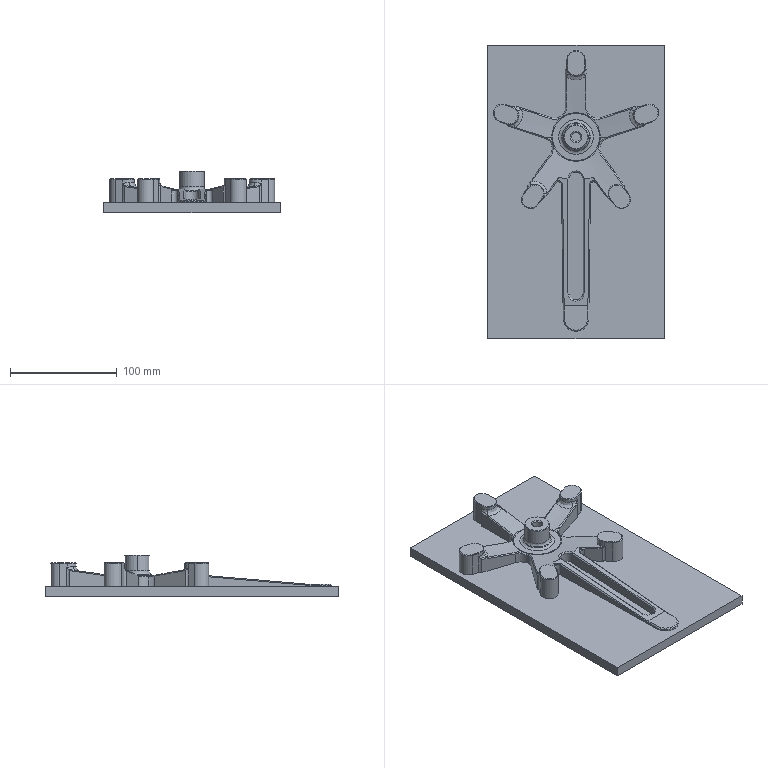NC program | NX | posted with a generic post | part box 165 x 275 x 39 mm
Lines 19900 to 20796 of 70117:
(CORNER_ROUGH , TOOL : D6)
N39798 M6
N39800 G54
N39802 G17 G0 G90 X70.448 Y9.221 S0 M3
N39804 G43 Z30. H0
N39806 Z-13.078
N39808 G94 G1 X69.985 Y10.648 F250.
N39810 X67.131 Y9.721
N39812 X66.147 Y9.401
N39814 G2 X65.321 Y8.792 R3.025
N39816 G1 X60.728 Y6.494
N39818 G0 X70.664 Y9.291 Z-13.572
N39820 G1 X70.2 Y10.718
N39822 X67.347 Y9.791
N39824 X66.147 Y9.401
N39826 G2 X65.327 Y8.558 R2.815
N39828 G1 X61.733 Y6.16
N39830 G0 X70.931 Y9.378 Z-14.066
N39832 G1 X70.467 Y10.804
N39834 X67.614 Y9.877
N39836 X66.146 Y9.4
N39838 G2 X65.375 Y8.263 R2.984
N39840 G1 X62.698 Y5.807
N39842 G0 X70.594 Y8.181 Z-14.56
N39844 G1 X67.799 Y9.271
N39846 G3 X67.818 Y9.944 R1.
N39848 G1 X66.111 Y9.389
N39850 G2 X66.077 Y9.14 R0.751
N39852 X65.455 Y8.04 R3.035
N39854 G3 X66.764 Y8.26 R1.
N39856 G2 X67.358 Y8.763 R2.06
N39858 G3 X67.799 Y9.271 R1.
N39860 G1 X70.594 Y8.181
N39862 G0 Y8.18 Z-15.054
N39864 G1 X67.799 Y9.271
N39866 G3 X67.819 Y9.944 R1.
N39868 G1 X66.111 Y9.389
N39870 G2 X66.077 Y9.14 R0.752
N39872 X65.454 Y8.039 R3.034
N39874 G3 X66.764 Y8.26 R1.
N39876 G2 X67.358 Y8.763 R2.06
N39878 G3 X67.799 Y9.271 R1.
N39880 G1 X70.594 Y8.18
N39882 G0 Y8.179 Z-15.548
N39884 G1 X67.799 Y9.271
N39886 G3 X67.819 Y9.944 R1.
N39888 G1 X66.111 Y9.389
N39890 G2 X66.077 Y9.14 R0.752
N39892 X65.454 Y8.039 R3.033
N39894 G3 X66.764 Y8.26 R1.
N39896 G2 X67.358 Y8.763 R2.06
N39898 G3 X67.799 Y9.271 R1.
N39900 G1 X70.594 Y8.179
N39902 G0 Z-16.042
N39904 G1 X67.799 Y9.271
N39906 G3 X67.819 Y9.944 R1.
N39908 G1 X66.111 Y9.389
N39910 G2 X66.077 Y9.14 R0.753
N39912 X65.454 Y8.039 R3.032
N39914 G3 X66.764 Y8.26 R1.
N39916 G2 X67.358 Y8.763 R2.06
N39918 G3 X67.799 Y9.271 R1.
N39920 G1 X70.594 Y8.179
N39922 G0 Y8.178 Z-16.536
N39924 G1 X67.8 Y9.271
N39926 G3 X67.819 Y9.944 R1.
N39928 G1 X66.111 Y9.389
N39930 G2 X66.077 Y9.14 R0.753
N39932 X65.454 Y8.038 R3.03
N39934 G3 X66.764 Y8.259 R1.
N39936 G2 X67.359 Y8.764 R2.06
N39938 G3 X67.8 Y9.271 R1.
N39940 G1 X70.594 Y8.178
N39942 G0 Z-17.03
N39944 G1 X67.8 Y9.271
N39946 G3 X67.82 Y9.944 R1.
N39948 G1 X66.111 Y9.389
N39950 G2 X66.077 Y9.14 R0.754
N39952 X65.454 Y8.038 R3.029
N39954 G3 X66.764 Y8.259 R1.
N39956 G2 X67.359 Y8.764 R2.06
N39958 G3 X67.8 Y9.271 R1.
N39960 G1 X70.594 Y8.178
N39962 G0 Y8.177 Z-17.524
N39964 G1 X67.8 Y9.271
N39966 G3 X67.82 Y9.944 R1.
N39968 G1 X66.111 Y9.389
N39970 G2 X66.077 Y9.14 R0.754
N39972 X65.454 Y8.038 R3.028
N39974 G3 X66.764 Y8.259 R1.
N39976 G2 X67.359 Y8.764 R2.06
N39978 G3 X67.8 Y9.271 R1.
N39980 G1 X70.594 Y8.177
N39982 G0 Z-18.018
N39984 G1 X67.8 Y9.271
N39986 G3 X67.82 Y9.944 R1.
N39988 G1 X66.111 Y9.389
N39990 G2 X66.077 Y9.141 R0.755
N39992 X65.454 Y8.037 R3.027
N39994 G3 X66.764 Y8.259 R1.
N39996 G2 X67.36 Y8.764 R2.06
N39998 G3 X67.8 Y9.271 R1.
N40000 G1 X70.594 Y8.177
N40002 G0 Y8.176 Z-18.512
N40004 G1 X67.8 Y9.271
N40006 G3 X67.82 Y9.944 R1.
N40008 G1 X66.111 Y9.389
N40010 G2 X66.077 Y9.141 R0.755
N40012 X65.454 Y8.037 R3.026
N40014 G3 X66.764 Y8.259 R1.
N40016 G2 X67.36 Y8.764 R2.06
N40018 G3 X67.8 Y9.271 R1.
N40020 G1 X70.594 Y8.176
N40022 G0 Y8.175 Z-19.006
N40024 G1 X67.801 Y9.27
N40026 G3 X67.821 Y9.944 R1.
N40028 G1 X66.111 Y9.389
N40030 G2 X66.077 Y9.141 R0.756
N40032 X65.454 Y8.037 R3.025
N40034 G3 X66.764 Y8.258 R1.
N40036 G2 X67.36 Y8.764 R2.06
N40038 G3 X67.801 Y9.27 R1.
N40040 G1 X70.594 Y8.175
N40042 G0 Z-19.5
N40044 G1 X67.801 Y9.27
N40046 G3 X67.821 Y9.945 R1.
N40048 G1 X66.111 Y9.389
N40050 G2 X66.078 Y9.143 R0.749
N40052 X65.454 Y8.037 R3.02
N40054 G3 X66.764 Y8.258 R1.
N40056 G2 X67.36 Y8.764 R2.06
N40058 G3 X67.801 Y9.27 R1.
N40060 G1 X70.594 Y8.175
N40062 G0 Y8.174 Z-20.
N40064 G1 X67.801 Y9.27
N40066 G3 X67.821 Y9.945 R1.
N40068 G1 X66.111 Y9.389
N40070 G2 X66.078 Y9.143 R0.749
N40072 X65.454 Y8.036 R3.019
N40074 G3 X66.764 Y8.258 R1.
N40076 G2 X67.361 Y8.764 R2.06
N40078 G3 X67.801 Y9.27 R1.
N40080 G1 X70.594 Y8.174
N40082 G0 Z-20.5
N40084 G1 X67.801 Y9.27
N40086 G3 X67.822 Y9.945 R1.
N40088 G1 X66.111 Y9.389
N40090 G2 X66.078 Y9.143 R0.75
N40092 X65.454 Y8.036 R3.018
N40094 G3 X66.764 Y8.258 R1.
N40096 G2 X67.361 Y8.764 R2.06
N40098 G3 X67.801 Y9.27 R1.
N40100 G1 X70.594 Y8.174
N40102 G0 Y8.173 Z-21.
N40104 G1 X67.801 Y9.27
N40106 G3 X67.822 Y9.945 R1.
N40108 G1 X66.111 Y9.389
N40110 G2 X66.078 Y9.143 R0.751
N40112 X65.454 Y8.036 R3.016
N40114 G3 X66.764 Y8.258 R1.
N40116 G2 X67.361 Y8.764 R2.06
N40118 G3 X67.801 Y9.27 R1.
N40120 G1 X70.594 Y8.173
N40122 G0 Z-21.5
N40124 G1 X67.802 Y9.27
N40126 G3 X67.822 Y9.945 R1.
N40128 G1 X66.111 Y9.389
N40130 G2 X66.078 Y9.143 R0.751
N40132 X65.454 Y8.035 R3.015
N40134 G3 X66.764 Y8.258 R1.
N40136 G2 X67.361 Y8.764 R2.06
N40138 G3 X67.802 Y9.27 R1.
N40140 G1 X70.594 Y8.173
N40142 G0 Y8.172 Z-22.
N40144 G1 X67.802 Y9.27
N40146 G3 X67.822 Y9.945 R1.
N40148 G1 X66.111 Y9.389
N40150 G2 X66.078 Y9.143 R0.752
N40152 X65.454 Y8.035 R3.014
N40154 G3 X66.764 Y8.257 R1.
N40156 G2 X67.362 Y8.764 R2.06
N40158 G3 X67.802 Y9.27 R1.
N40160 G1 X70.594 Y8.172
N40162 G0 Y8.171 Z-22.5
N40164 G1 X67.802 Y9.27
N40166 G3 X67.823 Y9.945 R1.
N40168 G1 X66.111 Y9.389
N40170 G2 X66.078 Y9.143 R0.753
N40172 X65.454 Y8.035 R3.013
N40174 G3 X66.764 Y8.257 R1.
N40176 G2 X67.362 Y8.765 R2.06
N40178 G3 X67.802 Y9.27 R1.
N40180 G1 X70.594 Y8.171
N40182 G0 Z-23.
N40184 G1 X67.802 Y9.27
N40186 G3 X67.823 Y9.945 R1.
N40188 G1 X66.111 Y9.389
N40190 G2 X66.078 Y9.143 R0.753
N40192 X65.454 Y8.034 R3.012
N40194 G3 X66.764 Y8.257 R1.
N40196 G2 X67.362 Y8.765 R2.06
N40198 G3 X67.802 Y9.27 R1.
N40200 G1 X70.594 Y8.171
N40202 G0 Y8.17 Z-23.5
N40204 G1 X67.802 Y9.27
N40206 G3 X67.823 Y9.945 R1.
N40208 G1 X66.111 Y9.389
N40210 G2 X66.078 Y9.143 R0.754
N40212 X65.454 Y8.034 R3.01
N40214 G3 X66.764 Y8.257 R1.
N40216 G2 X67.362 Y8.765 R2.06
N40218 G3 X67.802 Y9.27 R1.
N40220 G1 X70.594 Y8.17
N40222 G0 Z-24.
N40224 G1 X67.803 Y9.27
N40226 G3 X67.823 Y9.945 R1.
N40228 G1 X66.111 Y9.389
N40230 G2 X66.078 Y9.143 R0.755
N40232 X65.454 Y8.034 R3.009
N40234 G3 X66.765 Y8.257 R1.
N40236 G2 X67.363 Y8.765 R2.06
N40238 G3 X67.803 Y9.27 R1.
N40240 G1 X70.594 Y8.17
N40242 G0 Y8.169 Z-24.5
N40244 G1 X67.803 Y9.27
N40246 G3 X67.824 Y9.945 R1.
N40248 G1 X66.111 Y9.389
N40250 G2 X66.078 Y9.143 R0.755
N40252 X65.453 Y8.033 R3.008
N40254 G3 X66.765 Y8.256 R1.
N40256 G2 X67.363 Y8.765 R2.06
N40258 G3 X67.803 Y9.27 R1.
N40260 G1 X70.594 Y8.169
N40262 G0 Y8.168 Z-25.
N40264 G1 X67.803 Y9.269
N40266 G3 X67.824 Y9.946 R1.
N40268 G1 X66.111 Y9.389
N40270 G2 X66.078 Y9.143 R0.756
N40272 X65.453 Y8.033 R3.007
N40274 G3 X66.765 Y8.256 R1.
N40276 G2 X67.363 Y8.765 R2.06
N40278 G3 X67.803 Y9.269 R1.
N40280 G1 X70.594 Y8.168
N40282 G0 Z-25.5
N40284 G1 X67.803 Y9.269
N40286 G3 X67.824 Y9.946 R1.
N40288 G1 X66.111 Y9.389
N40290 X66.125 Y9.314
N40292 G2 X65.453 Y8.032 R3.006
N40294 G3 X66.764 Y8.256 R1.
N40296 G2 X67.364 Y8.765 R2.06
N40298 G3 X67.803 Y9.269 R1.
N40300 G1 X70.594 Y8.168
N40302 G0 Y8.167 Z-26.
N40304 G1 X67.803 Y9.269
N40306 G3 X67.824 Y9.946 R1.
N40308 G1 X66.111 Y9.389
N40310 X66.125 Y9.314
N40312 X66.071 Y9.121
N40314 G2 X65.453 Y8.032 R3.004
N40316 G3 X66.765 Y8.256 R1.
N40318 G2 X67.364 Y8.765 R2.06
N40320 G3 X67.803 Y9.269 R1.
N40322 G1 X70.594 Y8.167
N40324 G0 Z-26.5
N40326 G1 X67.804 Y9.269
N40328 G3 X67.825 Y9.946 R1.
N40330 G1 X66.111 Y9.389
N40332 X66.125 Y9.314
N40334 X66.071 Y9.121
N40336 G2 X65.453 Y8.032 R3.003
N40338 G3 X66.765 Y8.256 R1.
N40340 G2 X67.364 Y8.765 R2.06
N40342 G3 X67.804 Y9.269 R1.
N40344 G1 X70.594 Y8.167
N40346 G0 Y8.166 Z-27.
N40348 G1 X67.804 Y9.269
N40350 G3 X67.825 Y9.946 R1.
N40352 G1 X66.111 Y9.389
N40354 X66.126 Y9.314
N40356 X66.071 Y9.121
N40358 G2 X65.453 Y8.032 R3.002
N40360 G3 X66.765 Y8.255 R1.
N40362 G2 X67.364 Y8.765 R2.06
N40364 G3 X67.804 Y9.269 R1.
N40366 G1 X70.594 Y8.166
N40368 G0 Z-27.5
N40370 G1 X67.804 Y9.269
N40372 G3 X67.825 Y9.946 R1.
N40374 G1 X66.111 Y9.389
N40376 X66.126 Y9.314
N40378 X66.071 Y9.121
N40380 G2 X65.453 Y8.031 R3.001
N40382 G3 X66.765 Y8.255 R1.
N40384 G2 X67.365 Y8.765 R2.06
N40386 G3 X67.804 Y9.269 R1.
N40388 G1 X70.594 Y8.166
N40390 G0 Y8.165 Z-28.
N40392 G1 X67.804 Y9.269
N40394 G3 X67.826 Y9.946 R1.
N40396 G1 X66.111 Y9.389
N40398 X66.126 Y9.314
N40400 X66.071 Y9.121
N40402 G2 X65.453 Y8.031 R3.
N40404 G3 X66.765 Y8.255 R1.
N40406 G2 X67.365 Y8.766 R2.06
N40408 G3 X67.804 Y9.269 R1.
N40410 G1 X70.594 Y8.165
N40412 G0 Y8.164 Z-28.5
N40414 G1 X67.805 Y9.269
N40416 G3 X67.826 Y9.946 R1.
N40418 G1 X66.111 Y9.389
N40420 X66.126 Y9.314
N40422 X66.071 Y9.121
N40424 G2 X65.453 Y8.031 R2.999
N40426 G3 X66.765 Y8.255 R1.
N40428 G2 X67.365 Y8.766 R2.06
N40430 G3 X67.805 Y9.269 R1.
N40432 G1 X70.594 Y8.164
N40434 G0 Z-29.
N40436 G1 X67.805 Y9.269
N40438 G3 X67.826 Y9.946 R1.
N40440 G1 X66.111 Y9.389
N40442 X66.126 Y9.314
N40444 X66.071 Y9.121
N40446 G2 X65.453 Y8.03 R2.997
N40448 G3 X66.765 Y8.255 R1.
N40450 G2 X67.365 Y8.766 R2.06
N40452 G3 X67.805 Y9.269 R1.
N40454 G1 X70.594 Y8.164
N40456 G0 Y8.163 Z-29.5
N40458 G1 X67.805 Y9.269
N40460 G3 X67.826 Y9.946 R1.
N40462 G1 X66.111 Y9.389
N40464 X66.127 Y9.314
N40466 X66.071 Y9.121
N40468 G2 X65.453 Y8.03 R2.996
N40470 G3 X66.765 Y8.254 R1.
N40472 G2 X67.366 Y8.766 R2.06
N40474 G3 X67.805 Y9.269 R1.
N40476 G1 X70.594 Y8.163
N40478 G0 Z3.
N40480 X58.601 Y35.255
N40482 Z-13.078
N40484 G1 X58.93 Y32.273
N40486 X58.919 Y32.272
N40488 G3 X58.023 Y31.288 R1.
N40490 G2 X59.037 Y31.274 R2.919
N40492 G1 X60.009 Y31.59
N40494 G3 X58.942 Y32.274 R1.
N40496 G1 X58.93 Y32.273
N40498 X58.601 Y35.255
N40500 G0 X58.932 Y35.334 Z-13.572
N40502 G1 X58.93 Y32.334
N40504 X58.905 Y32.335
N40506 G3 X57.9 Y31.461 R1.
N40508 G2 X59.066 Y31.283 R3.722
N40510 G1 X60.236 Y31.664
N40512 G3 X59.17 Y32.348 R1.
N40514 G2 X58.93 Y32.334 R2.06
N40516 G1 X58.932 Y35.334
N40518 G0 X59.321 Y35.415 Z-14.066
N40520 G1 X58.944 Y32.439
N40522 X58.86 Y32.451
N40524 G3 X57.731 Y31.734 R1.
N40526 G2 X59.04 Y31.275 R3.047
N40528 G1 X60.508 Y31.752
N40530 G3 X59.441 Y32.436 R1.
N40532 G2 X58.944 Y32.439 R2.06
N40534 G1 X59.321 Y35.415
N40536 G0 X54.17 Y32.743 Z-14.56
N40538 G1 X57.673 Y31.975
N40540 G2 X58.971 Y31.332 R3.
N40542 G1 X59.04 Y31.275
N40544 X60.718 Y31.82
N40546 X63.571 Y32.747
N40548 X63.108 Y34.174
N40550 G0 X53.979 Y32.785 Z-15.054
N40552 G1 X57.673 Y31.975
N40554 G2 X58.971 Y31.332 R3.
N40556 G1 X59.04 Y31.275
N40558 X60.718 Y31.82
N40560 X63.571 Y32.747
N40562 X63.108 Y34.174
N40564 G0 X53.979 Y32.785 Z-15.548
N40566 G1 X57.673 Y31.975
N40568 G2 X58.971 Y31.332 R3.
N40570 G1 X59.04 Y31.275
N40572 X60.718 Y31.82
N40574 X63.571 Y32.747
N40576 X63.108 Y34.174
N40578 G0 X53.979 Y32.785 Z-16.042
N40580 G1 X57.673 Y31.975
N40582 G2 X58.971 Y31.332 R3.
N40584 G1 X59.04 Y31.275
N40586 X60.718 Y31.82
N40588 X63.571 Y32.747
N40590 X63.108 Y34.174
N40592 G0 X53.979 Y32.785 Z-16.536
N40594 G1 X57.673 Y31.975
N40596 G2 X58.971 Y31.332 R3.
N40598 G1 X59.04 Y31.275
N40600 X60.718 Y31.82
N40602 X63.571 Y32.747
N40604 X63.108 Y34.174
N40606 G0 X53.979 Y32.785 Z-17.03
N40608 G1 X57.673 Y31.975
N40610 G2 X58.971 Y31.332 R3.
N40612 G1 X59.04 Y31.275
N40614 X60.718 Y31.82
N40616 X63.571 Y32.747
N40618 X63.108 Y34.174
N40620 G0 X53.979 Y32.785 Z-17.524
N40622 G1 X57.673 Y31.975
N40624 G2 X58.971 Y31.332 R3.
N40626 G1 X59.04 Y31.275
N40628 X60.718 Y31.82
N40630 X63.571 Y32.747
N40632 X63.108 Y34.174
N40634 G0 X53.979 Y32.785 Z-18.018
N40636 G1 X57.673 Y31.975
N40638 G2 X58.971 Y31.332 R3.
N40640 G1 X59.04 Y31.275
N40642 X60.718 Y31.82
N40644 X63.571 Y32.747
N40646 X63.108 Y34.174
N40648 G0 X53.979 Y32.785 Z-18.512
N40650 G1 X57.673 Y31.975
N40652 G2 X58.971 Y31.332 R3.
N40654 G1 X59.04 Y31.275
N40656 X60.718 Y31.82
N40658 X63.571 Y32.747
N40660 X63.108 Y34.174
N40662 G0 X59.618 Y35.468 Z-19.006
N40664 G1 X58.966 Y32.54
N40666 X58.866 Y32.565
N40668 G3 X57.673 Y31.975 R1.
N40670 G2 X58.971 Y31.332 R3.
N40672 G1 X59.04 Y31.275
N40674 X60.718 Y31.82
N40676 G3 X59.652 Y32.505 R1.
N40678 G2 X58.966 Y32.54 R2.06
N40680 G1 X59.618 Y35.468
N40682 G0 Z-19.5
N40684 G1 X58.966 Y32.54
N40686 X58.866 Y32.565
N40688 G3 X57.673 Y31.975 R1.
N40690 G2 X58.971 Y31.332 R3.
N40692 G1 X59.04 Y31.275
N40694 X60.718 Y31.82
N40696 G3 X59.652 Y32.505 R1.
N40698 G2 X58.966 Y32.54 R2.06
N40700 G1 X59.618 Y35.468
N40702 G0 Z-20.
N40704 G1 X58.966 Y32.54
N40706 X58.866 Y32.565
N40708 G3 X57.673 Y31.975 R1.
N40710 G2 X58.971 Y31.332 R3.
N40712 G1 X59.04 Y31.275
N40714 X60.718 Y31.82
N40716 G3 X59.652 Y32.505 R1.
N40718 G2 X58.966 Y32.54 R2.06
N40720 G1 X59.618 Y35.468
N40722 G0 Z-20.5
N40724 G1 X58.966 Y32.54
N40726 X58.866 Y32.565
N40728 G3 X57.673 Y31.975 R1.
N40730 G2 X58.971 Y31.332 R3.
N40732 G1 X59.04 Y31.275
N40734 X60.718 Y31.82
N40736 G3 X59.652 Y32.505 R1.
N40738 G2 X58.966 Y32.54 R2.06
N40740 G1 X59.618 Y35.468
N40742 G0 Z-21.
N40744 G1 X58.966 Y32.54
N40746 X58.866 Y32.565
N40748 G3 X57.673 Y31.975 R1.
N40750 G2 X58.971 Y31.332 R3.
N40752 G1 X59.04 Y31.275
N40754 X60.718 Y31.82
N40756 G3 X59.652 Y32.505 R1.
N40758 G2 X58.966 Y32.54 R2.06
N40760 G1 X59.618 Y35.468
N40762 G0 Z-21.5
N40764 G1 X58.966 Y32.54
N40766 X58.866 Y32.565
N40768 G3 X57.673 Y31.975 R1.
N40770 G2 X58.971 Y31.332 R3.
N40772 G1 X59.04 Y31.275
N40774 X60.718 Y31.82
N40776 G3 X59.652 Y32.505 R1.
N40778 G2 X58.966 Y32.54 R2.06
N40780 G1 X59.618 Y35.468
N40782 G0 Z-22.
N40784 G1 X58.966 Y32.54
N40786 X58.866 Y32.565
N40788 G3 X57.673 Y31.975 R1.
N40790 G2 X58.971 Y31.332 R3.
N40792 G1 X59.04 Y31.275
N40794 X60.718 Y31.82
N40796 G3 X59.652 Y32.505 R1.
N40798 G2 X58.966 Y32.54 R2.06
N40800 G1 X59.618 Y35.468
N40802 G0 Z-22.5
N40804 G1 X58.966 Y32.54
N40806 X58.866 Y32.565
N40808 G3 X57.673 Y31.975 R1.
N40810 G2 X58.971 Y31.332 R3.
N40812 G1 X59.04 Y31.275
N40814 X60.718 Y31.82
N40816 G3 X59.652 Y32.505 R1.
N40818 G2 X58.966 Y32.54 R2.06
N40820 G1 X59.618 Y35.468
N40822 G0 Z-23.
N40824 G1 X58.966 Y32.54
N40826 X58.866 Y32.565
N40828 G3 X57.673 Y31.975 R1.
N40830 G2 X58.971 Y31.332 R3.
N40832 G1 X59.04 Y31.275
N40834 X60.718 Y31.82
N40836 G3 X59.652 Y32.505 R1.
N40838 G2 X58.966 Y32.54 R2.06
N40840 G1 X59.618 Y35.468
N40842 G0 Z-23.5
N40844 G1 X58.966 Y32.54
N40846 X58.866 Y32.565
N40848 G3 X57.673 Y31.975 R1.
N40850 G2 X58.971 Y31.332 R3.
N40852 G1 X59.04 Y31.275
N40854 X60.718 Y31.82
N40856 G3 X59.652 Y32.505 R1.
N40858 G2 X58.966 Y32.54 R2.06
N40860 G1 X59.618 Y35.468
N40862 G0 Z-24.
N40864 G1 X58.966 Y32.54
N40866 X58.866 Y32.565
N40868 G3 X57.673 Y31.975 R1.
N40870 G2 X58.971 Y31.332 R3.
N40872 G1 X59.04 Y31.275
N40874 X60.718 Y31.82
N40876 G3 X59.652 Y32.505 R1.
N40878 G2 X58.966 Y32.54 R2.06
N40880 G1 X59.618 Y35.468
N40882 G0 Z-24.5
N40884 G1 X58.966 Y32.54
N40886 X58.866 Y32.565
N40888 G3 X57.673 Y31.975 R1.
N40890 G2 X58.971 Y31.332 R3.
N40892 G1 X59.04 Y31.275
N40894 X60.718 Y31.82
N40896 G3 X59.652 Y32.505 R1.
N40898 G2 X58.966 Y32.54 R2.06
N40900 G1 X59.618 Y35.468
N40902 G0 Z-25.
N40904 G1 X58.966 Y32.54
N40906 X58.866 Y32.565
N40908 G3 X57.673 Y31.975 R1.
N40910 G2 X58.971 Y31.332 R3.
N40912 G1 X59.04 Y31.275
N40914 X60.718 Y31.82
N40916 G3 X59.652 Y32.505 R1.
N40918 G2 X58.966 Y32.54 R2.06
N40920 G1 X59.618 Y35.468
N40922 G0 Z-25.5
N40924 G1 X58.966 Y32.54
N40926 X58.866 Y32.565
N40928 G3 X57.673 Y31.975 R1.
N40930 G2 X58.971 Y31.332 R3.
N40932 G1 X59.04 Y31.275
N40934 X60.718 Y31.82
N40936 G3 X59.652 Y32.505 R1.
N40938 G2 X58.966 Y32.54 R2.06
N40940 G1 X59.618 Y35.468
N40942 G0 Z-26.
N40944 G1 X58.966 Y32.54
N40946 X58.866 Y32.565
N40948 G3 X57.673 Y31.975 R1.
N40950 G2 X58.971 Y31.332 R3.
N40952 G1 X59.04 Y31.275
N40954 X60.718 Y31.82
N40956 G3 X59.652 Y32.505 R1.
N40958 G2 X58.966 Y32.54 R2.06
N40960 G1 X59.618 Y35.468
N40962 G0 Z-26.5
N40964 G1 X58.966 Y32.54
N40966 X58.866 Y32.565
N40968 G3 X57.673 Y31.975 R1.
N40970 G2 X58.971 Y31.332 R3.
N40972 G1 X59.04 Y31.275
N40974 X60.718 Y31.82
N40976 G3 X59.652 Y32.505 R1.
N40978 G2 X58.966 Y32.54 R2.06
N40980 G1 X59.618 Y35.468
N40982 G0 Z-27.
N40984 G1 X58.966 Y32.54
N40986 X58.866 Y32.565
N40988 G3 X57.673 Y31.975 R1.
N40990 G2 X58.971 Y31.332 R3.
N40992 G1 X59.04 Y31.275
N40994 X60.718 Y31.82
N40996 G3 X59.652 Y32.505 R1.
N40998 G2 X58.966 Y32.54 R2.06
N41000 G1 X59.618 Y35.468
N41002 G0 Z-27.5
N41004 G1 X58.966 Y32.54
N41006 X58.866 Y32.565
N41008 G3 X57.673 Y31.975 R1.
N41010 G2 X58.971 Y31.332 R3.
N41012 G1 X59.04 Y31.275
N41014 X60.718 Y31.82
N41016 G3 X59.652 Y32.505 R1.
N41018 G2 X58.966 Y32.54 R2.06
N41020 G1 X59.618 Y35.468
N41022 G0 Z-28.
N41024 G1 X58.966 Y32.54
N41026 X58.866 Y32.565
N41028 G3 X57.673 Y31.975 R1.
N41030 G2 X58.971 Y31.332 R3.
N41032 G1 X59.04 Y31.275
N41034 X60.718 Y31.82
N41036 G3 X59.652 Y32.505 R1.
N41038 G2 X58.966 Y32.54 R2.06
N41040 G1 X59.618 Y35.468
N41042 G0 Z-28.5
N41044 G1 X58.966 Y32.54
N41046 X58.866 Y32.565
N41048 G3 X57.673 Y31.975 R1.
N41050 G2 X58.971 Y31.332 R3.
N41052 G1 X59.04 Y31.275
N41054 X60.718 Y31.82
N41056 G3 X59.652 Y32.505 R1.
N41058 G2 X58.966 Y32.54 R2.06
N41060 G1 X59.618 Y35.468
N41062 G0 Z-29.
N41064 G1 X58.966 Y32.54
N41066 X58.866 Y32.565
N41068 G3 X57.673 Y31.975 R1.
N41070 G2 X58.971 Y31.332 R3.
N41072 G1 X59.04 Y31.275
N41074 X60.718 Y31.82
N41076 G3 X59.652 Y32.505 R1.
N41078 G2 X58.966 Y32.54 R2.06
N41080 G1 X59.618 Y35.468
N41082 G0 Z-29.5
N41084 G1 X58.966 Y32.54
N41086 X58.866 Y32.565
N41088 G3 X57.673 Y31.975 R1.
N41090 G2 X58.971 Y31.332 R3.
N41092 G1 X59.04 Y31.275
N41094 X60.718 Y31.82
N41096 G3 X59.652 Y32.505 R1.
N41098 G2 X58.966 Y32.54 R2.06
N41100 G1 X59.618 Y35.468
N41102 G0 Z-10.078
N41104 X20.044 Y-2.408
N41106 Z-19.006
N41108 G1 X20.038 Y1.492
N41110 G2 X20.467 Y1.472 R4.46
N41112 G3 X17.425 Y10.838 R20.52
N41114 G2 X16.729 Y10.334 R4.46
N41116 X19.608 Y1.47 R19.663
N41118 X20.038 Y1.492 R4.46
N41120 G1 X20.04 Y0.292
N41122 G2 X21.719 Y-0.171 R3.26
N41124 G3 X17.472 Y12.903 R21.72
N41126 G2 X14.869 Y10.946 R3.26
N41128 X18.463 Y-0.118 R18.463
N41130 X20.04 Y0.292 R3.26
N41132 G1 X20.042 Y-0.908
N41134 G2 X21.953 Y-2.192 R2.06
N41136 G3 X23.124 Y-2.785 R1.
N41138 G2 X22.877 Y-1.411 R2.946
N41140 G3 X17.706 Y14.555 R22.92
N41142 G2 X17.081 Y15.868 R3.009
N41144 G3 X16.47 Y14.689 R1.
N41146 G2 X13.289 Y12.496 R2.06
N41148 G3 X12.016 Y12.395 R1.
N41150 G2 X17.007 Y-2.967 R17.263
N41152 G3 X18.096 Y-2.301 R1.
N41154 G2 X20.042 Y-0.908 R2.06
N41156 G1 X20.046 Y-3.908
N41158 G0 X17.642 Y-9.814
N41160 G1 X15.348 Y-12.968
N41162 G2 X15.013 Y-12.699 R4.46
N41164 X-15.012 Y-12.7 R19.663
N41166 X-15.707 Y-13.205 R4.46
N41168 G3 X15.708 Y-13.204 R20.52
N41170 G2 X15.348 Y-12.968 R4.46
N41172 G1 X16.054 Y-11.998
N41174 G2 X15.018 Y-10.741 R3.26
N41176 X-15.017 Y-10.742 R18.463
N41178 X-17.685 Y-12.61 R3.26
N41180 G3 X17.686 Y-12.609 R21.72
N41182 G2 X16.054 Y-11.998 R3.26
N41184 G1 X16.76 Y-11.027
N41186 G2 X16.002 Y-8.758 R2.06
N41188 G3 X15.511 Y-7.579 R1.
N41190 G2 X-15.51 Y-7.58 R17.263
N41192 G3 X-16.001 Y-8.759 R1.
N41194 G2 X-19.07 Y-11.105 R2.06
N41196 G3 X-20.38 Y-11.32 R1.
N41198 G2 X-19.333 Y-12.312 R2.962
N41200 G3 X19.266 Y-12.416 R22.92
N41202 G2 X20.387 Y-11.321 R2.993
N41204 G3 X19.073 Y-11.102 R1.
N41206 G2 X16.76 Y-11.027 R2.06
N41208 G1 X18.524 Y-8.601
N41210 G0 Z3.
N41212 X-20.044 Y-2.405
N41214 Z-19.006
N41216 G1 X-20.037 Y1.495
N41218 G2 X-19.608 Y1.474 R4.46
N41220 X-16.726 Y10.339 R19.663
N41222 X-17.421 Y10.843 R4.46
N41224 G3 X-20.467 Y1.475 R20.52
N41226 G2 X-20.037 Y1.495 R4.46
N41228 G1 X-20.04 Y0.295
N41230 G2 X-18.463 Y-0.114 R3.26
N41232 X-14.866 Y10.95 R18.463
N41234 X-17.468 Y12.908 R3.26
N41236 G3 X-21.72 Y0.008 R21.72
N41238 G1 X-21.719 Y-0.167
N41240 G2 X-20.04 Y0.295 R3.26
N41242 G1 X-20.042 Y-0.905
N41244 G2 X-18.096 Y-2.298 R2.06
N41246 G3 X-17.007 Y-2.964 R1.
N41248 G2 X-12.012 Y12.399 R17.263
N41250 G3 X-13.285 Y12.501 R1.
N41252 G2 X-16.468 Y14.684 R2.06
N41254 G3 X-17.07 Y15.855 R1.
N41256 G2 X-17.683 Y14.582 R2.965
N41258 G3 X-22.876 Y-1.412 R22.92
N41260 G2 X-23.119 Y-2.779 R2.95
N41262 G3 X-21.953 Y-2.186 R1.
N41264 G2 X-20.042 Y-0.905 R2.06
N41266 G1 X-20.047 Y-3.905
N41268 G0 Z-14.524
N41270 X-8.48 Y18.321
N41272 Z-19.006
N41274 G1 X-4.768 Y19.519
N41276 G2 X-4.656 Y19.104 R4.46
N41278 X4.661 Y19.103 R19.663
N41280 X4.925 Y19.92 R4.46
N41282 G3 X-4.92 Y19.921 R20.52
N41284 G2 X-4.768 Y19.519 R4.46
N41286 G1 X-5.91 Y19.151
N41288 G2 X-5.813 Y17.525 R3.26
N41290 X5.817 Y17.523 R18.463
N41292 X6.874 Y20.603 R3.26
N41294 G3 X-6.869 Y20.605 R21.72
N41296 G2 X-5.91 Y19.151 R3.26
N41298 G1 X-7.052 Y18.782
N41300 G2 X-7.776 Y16.501 R2.06
N41302 G3 X-8.073 Y15.26 R1.
N41304 G2 X8.077 Y15.258 R17.263
N41306 G3 X7.78 Y16.499 R1.
N41308 G2 X8.874 Y20.202 R2.06
N41310 G3 X9.803 Y21.139 R1.
N41312 G2 X8.394 Y21.328 R2.968
N41314 G3 X-8.399 Y21.326 R22.92
N41316 G2 X-9.792 Y21.135 R2.965
N41318 G3 X-8.866 Y20.204 R1.
N41320 G2 X-7.052 Y18.782 R2.06
N41322 G1 X-9.907 Y17.86
N41324 G0 X0. Y18.989 Z-16.006
N41326 G1 Z-19.5
N41328 G2 X18.989 Y0. R18.989
N41330 X0. Y18.989 R-18.989
N41332 G1 Y19.415
N41334 G3 X-19.415 Y0. R19.415
N41336 X0. Y19.415 R-19.415
N41338 G0 Z3.
N41340 X13. Y69.835
N41342 Z-13.078
N41344 G1 X11.5
N41346 Y66.835
N41348 Y65.816
N41350 G2 X11.828 Y64.857 R2.806
N41352 G1 X12.592 Y59.744
N41354 G0 X13. Y70.089 Z-13.572
N41356 G1 X11.5
N41358 Y67.089
N41360 Y65.815
N41362 G2 X12.052 Y64.762 R2.847
N41364 G1 X13.214 Y60.613
N41366 G0 X13. Y70.363 Z-14.066
N41368 G1 X11.5
N41370 Y67.363
N41372 Y65.797
N41374 G2 X12.359 Y64.703 R2.895
N41376 G1 X13.849 Y61.396
N41378 G0 X14.034 Y69.666 Z-14.56
N41380 G1 X12.134 Y67.345
N41382 G3 X11.5 Y67.572 R1.
N41384 G1 Y65.775
N41386 X11.66 Y65.713
N41388 G2 X12.581 Y64.733 R3.037
N41390 G3 X12.776 Y66.047 R1.
N41392 G2 X12.48 Y66.769 R2.06
N41394 G3 X12.134 Y67.345 R1.
N41396 G1 X14.034 Y69.666
N41398 G0 X14.035 Z-15.054
N41400 G1 X12.134 Y67.346
N41402 G3 X11.5 Y67.572 R1.
N41404 G1 Y65.775
N41406 X11.66 Y65.713
N41408 G2 X12.581 Y64.733 R3.036
N41410 G3 X12.776 Y66.047 R1.
N41412 G2 X12.48 Y66.769 R2.06
N41414 G3 X12.134 Y67.346 R1.
N41416 G1 X14.035 Y69.666
N41418 G0 X14.036 Z-15.548
N41420 G1 X12.134 Y67.346
N41422 G3 X11.5 Y67.572 R1.
N41424 G1 Y65.775
N41426 X11.66 Y65.713
N41428 G2 X12.581 Y64.733 R3.035
N41430 G3 X12.776 Y66.047 R1.
N41432 G2 X12.48 Y66.769 R2.06
N41434 G3 X12.134 Y67.346 R1.
N41436 G1 X14.036 Y69.666
N41438 G0 Z-16.042
N41440 G1 X12.134 Y67.346
N41442 G3 X11.5 Y67.573 R1.
N41444 G1 Y65.775
N41446 X11.66 Y65.713
N41448 G2 X12.582 Y64.733 R3.033
N41450 G3 X12.776 Y66.048 R1.
N41452 G2 X12.48 Y66.77 R2.06
N41454 G3 X12.134 Y67.346 R1.
N41456 G1 X14.036 Y69.666
N41458 G0 X14.037 Z-16.536
N41460 G1 X12.134 Y67.346
N41462 G3 X11.5 Y67.573 R1.
N41464 G1 Y65.775
N41466 X11.66 Y65.713
N41468 G2 X12.582 Y64.733 R3.032
N41470 G3 X12.776 Y66.048 R1.
N41472 G2 X12.48 Y66.77 R2.06
N41474 G3 X12.134 Y67.346 R1.
N41476 G1 X14.037 Y69.666
N41478 G0 Y69.665 Z-17.03
N41480 G1 X12.134 Y67.346
N41482 G3 X11.5 Y67.573 R1.
N41484 G1 Y65.775
N41486 X11.66 Y65.713
N41488 G2 X12.582 Y64.733 R3.031
N41490 G3 X12.777 Y66.048 R1.
N41492 G2 X12.48 Y66.77 R2.06
N41494 G3 X12.134 Y67.346 R1.
N41496 G1 X14.037 Y69.665
N41498 G0 X14.038 Z-17.524
N41500 G1 X12.134 Y67.346
N41502 G3 X11.5 Y67.573 R1.
N41504 G1 Y65.775
N41506 X11.66 Y65.713
N41508 G2 X12.582 Y64.733 R3.03
N41510 G3 X12.777 Y66.048 R1.
N41512 G2 X12.48 Y66.77 R2.06
N41514 G3 X12.134 Y67.346 R1.
N41516 G1 X14.038 Y69.665
N41518 G0 Z-18.018
N41520 G1 X12.135 Y67.347
N41522 G3 X11.5 Y67.574 R1.
N41524 G1 Y65.775
N41526 X11.66 Y65.713
N41528 G2 X12.582 Y64.733 R3.029
N41530 G3 X12.777 Y66.048 R1.
N41532 G2 X12.48 Y66.771 R2.06
N41534 G3 X12.135 Y67.347 R1.
N41536 G1 X14.038 Y69.665
N41538 G0 X14.039 Z-18.512
N41540 G1 X12.135 Y67.347
N41542 G3 X11.5 Y67.574 R1.
N41544 G1 Y65.775
N41546 X11.66 Y65.713
N41548 G2 X12.583 Y64.733 R3.027
N41550 G3 X12.777 Y66.048 R1.
N41552 G2 X12.48 Y66.771 R2.06
N41554 G3 X12.135 Y67.347 R1.
N41556 G1 X14.039 Y69.665
N41558 G0 Z-19.006
N41560 G1 X12.135 Y67.347
N41562 G3 X11.5 Y67.574 R1.
N41564 G1 Y65.775
N41566 X11.66 Y65.713
N41568 G2 X12.583 Y64.733 R3.026
N41570 G3 X12.777 Y66.048 R1.
N41572 G2 X12.48 Y66.771 R2.06
N41574 G3 X12.135 Y67.347 R1.
N41576 G1 X14.039 Y69.665
N41578 G0 X14.04 Z-19.5
N41580 G1 X12.135 Y67.347
N41582 G3 X11.5 Y67.574 R1.
N41584 G1 Y65.775